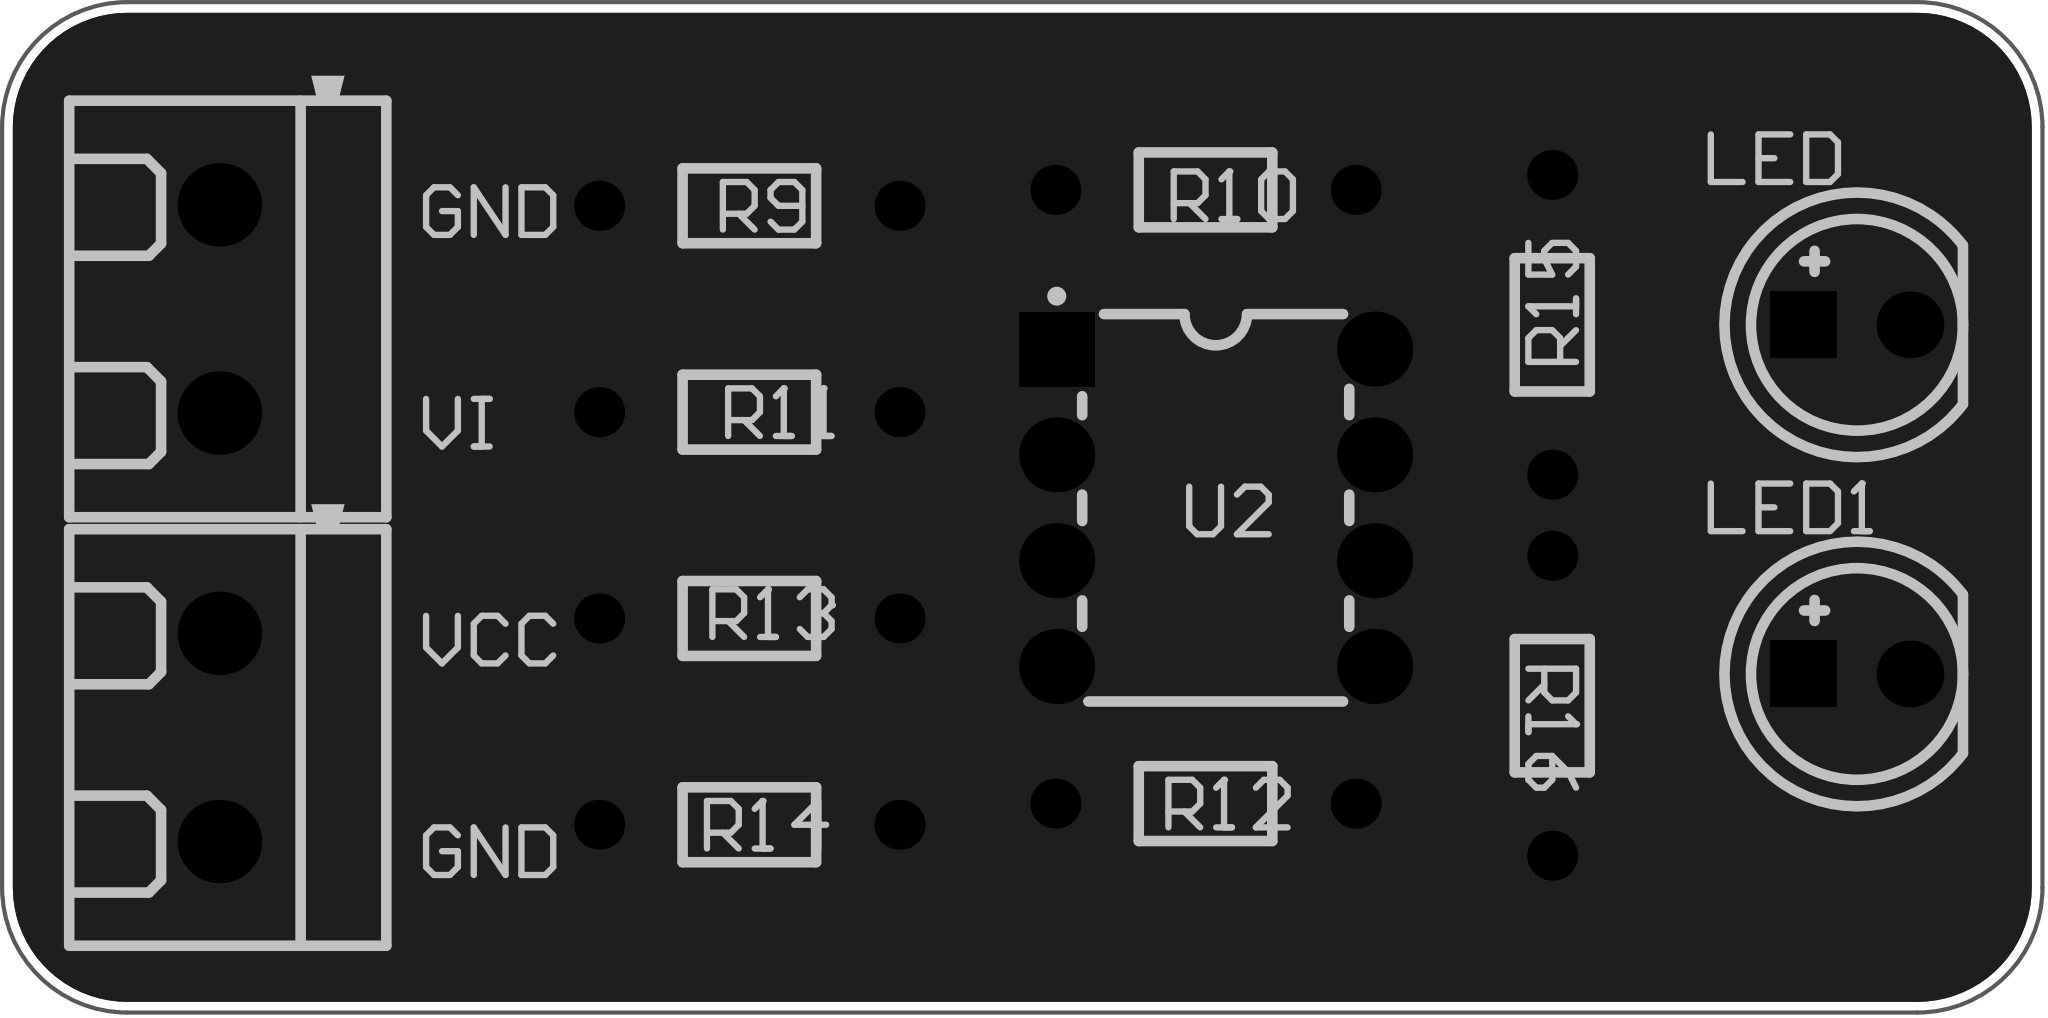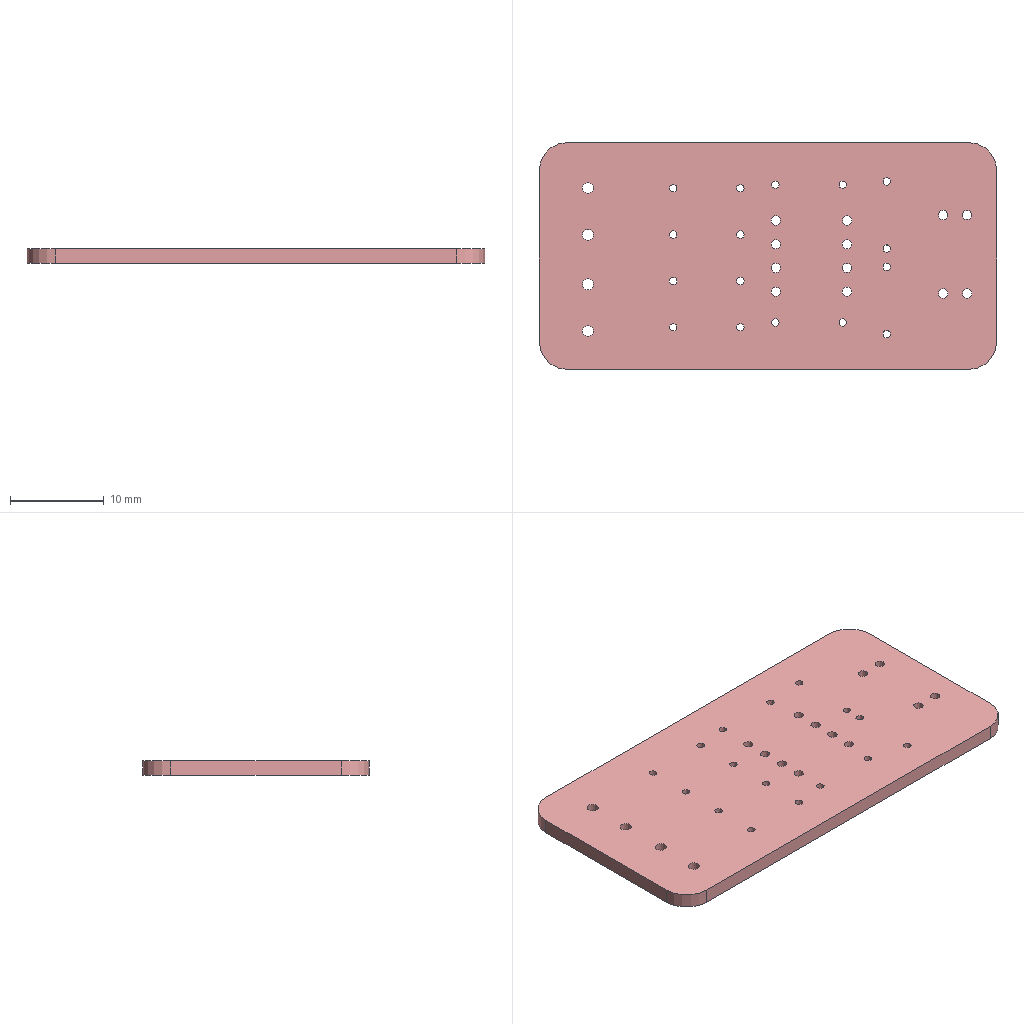Circuit board layout | Altium Designer | box 48.9 x 24.3 x 1.6 mm
Layer stack:
# Altium Designer layer stack of  (unit mm; dielectric type: 0 none, 1 core, 2 prepreg, 3 surface material)
index,name,kind,layer,copper_thickness_mm,dielectric_type,dielectric_thickness_mm,dielectric_material,dielectric_constant
0,Top Paste Mask Layer,other,,,,,,
1,Top Silkscreen Layer,other,,,,,,
2,Top Solder Mask Layer,dielectric,,,3,0.01,,3.3
3,Top Layer,copper,Top Layer,0.035,,,,
4,Dielectric1,dielectric,,,3,1.51,FR4,4.5
5,Bottom Layer,copper,Bottom Layer,0.035,,,,
6,Bottom Solder Mask Layer,dielectric,,,3,0.01,,3.3
7,Bottom Silkscreen Layer,other,,,,,,
8,Bottom Paste Mask Layer,other,,,,,,
# drill layer pairs: low layer,high layer
drill_pair,Top Layer,Bottom Layer
Part placement:
Designator,Comment,Layer,Footprint,Center-X(mm),Center-Y(mm),Rotation
LED,,TopLayer,LED-TH_5mm,124.714,94.996,0
LED1,,TopLayer,LED-TH_5mm,124.714,86.614,0
P1,KF301-2P接线端子,TopLayer,CONN-TH_XY301V-A-5.0-2P,85.471,85.09,90
P2,KF301-2P接线端子,TopLayer,CONN-TH_XY301V-A-5.0-2P,85.471,95.377,90
R9,30K,TopLayer,Res_1/8W,98.171,97.853,0
R10,68K,TopLayer,Res_1/8W,109.103,98.235,180
R11,30K,TopLayer,Res_1/8W,98.171,92.9,180
R12,68K,TopLayer,Res_1/8W,109.103,83.502,0
R13,51K,TopLayer,Res_1/8W,98.171,87.947,0
R14,13K,TopLayer,Res_1/8W,98.171,82.994,0
R15,220,TopLayer,Res_1/8W,117.411,94.996,90
R16,220,TopLayer,Res_1/8W,117.411,85.852,270
U2,LM324AD,TopLayer,DIP-8_L9.3-W6.4-P2.54-LS7.6-BL,109.347,90.603,270
Pad and via stacks:
# Altium Designer via and pad stacks of  (unit mm). Each distinct definition once, with the count of objects using it.
# via: kind,start_layer,end_layer,hole_mm,diameter_mm,mode(0 simple;1 top-mid-bottom;2 full stack),diameter_per_layer,count,example_net
# pad: kind,layer,hole_mm,hole_type(0 round;1 square;2 slot),plating,top_size,top_shape(1 round;2 rect;3 octagon;9 rounded rect),mid_size,bottom_size,mode,footprint,size_per_layer,count,example
pad,Multi-Layer,1,0,plated,1.6x1.6,2,1.6x1.6,1.6x1.6,0,LED-TH_5mm,,2,LED.1
pad,Multi-Layer,1,0,plated,1.6x1.6,1,1.6x1.6,1.6x1.6,0,LED-TH_5mm,,2,LED.2
pad,Multi-Layer,1.2,0,plated,2x2,1,2x2,2x2,0,CONN-TH_XY301V-A-5.0-2P,,4,P1.1
pad,Multi-Layer,0.8001,0,plated,1.199x1.199,1,1.199x1.199,1.199x1.199,0,Res_1/8W,,16,R9.1
pad,Multi-Layer,1,0,plated,1.8x1.8,2,1.8x1.8,1.8x1.8,0,DIP-8_L9.3-W6.4-P2.54-LS7.6-BL,,1,U2.1
pad,Multi-Layer,1,0,plated,1.8x1.8,1,1.8x1.8,1.8x1.8,0,DIP-8_L9.3-W6.4-P2.54-LS7.6-BL,,7,U2.2
Copper pours:
name,layer,net,type(0 solid;1 hatched;2 none)
Top Layer-GND,Top Layer,GND,0
Bottom Layer-GND,Bottom Layer,GND,0